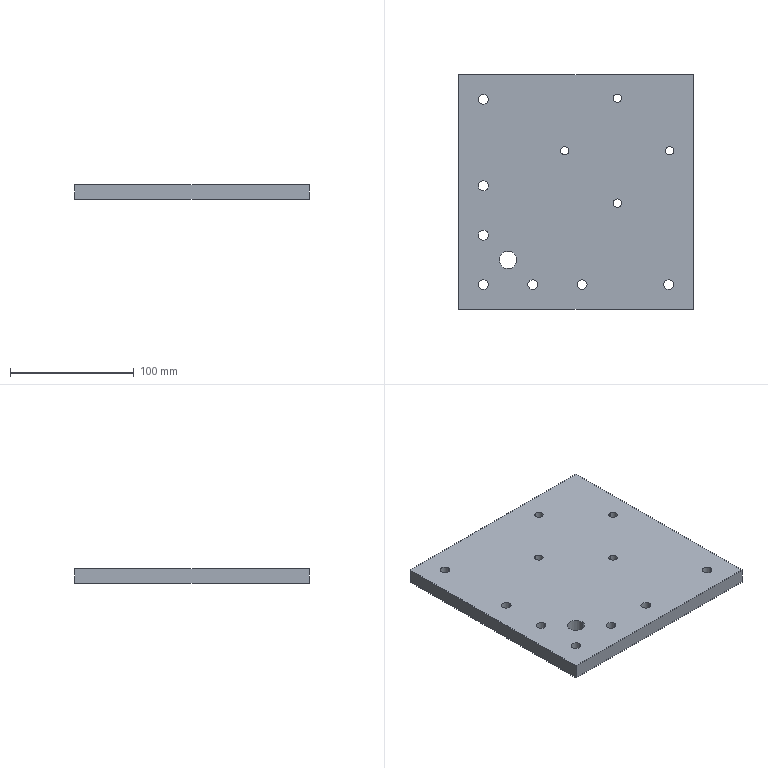Part | NX | 1 solid | 30 faces | box 190 x 190 x 12 mm | volume 425413 mm3 | cylinder 24 | plane 6 | commonest cylinder face diameters 8 x14 6.75 x8 14 x2
STEP:
#1=CARTESIAN_POINT('',(-95.,-95.,-6.));
#2=VERTEX_POINT('',#1);
#3=CARTESIAN_POINT('',(-95.,95.,-6.));
#4=VERTEX_POINT('',#3);
#5=CARTESIAN_POINT('',(-95.,-95.,-6.));
#6=DIRECTION('',(0.,1.,0.));
#7=VECTOR('',#6,1000.);
#8=LINE('',#5,#7);
#9=EDGE_CURVE('',#2,#4,#8,.T.);
#10=ORIENTED_EDGE('',*,*,#9,.T.);
#11=CARTESIAN_POINT('',(95.,95.,-6.));
#12=VERTEX_POINT('',#11);
#13=CARTESIAN_POINT('',(-95.,95.,-6.));
#14=DIRECTION('',(1.,0.,0.));
#15=VECTOR('',#14,1000.);
#16=LINE('',#13,#15);
#17=EDGE_CURVE('',#4,#12,#16,.T.);
#18=ORIENTED_EDGE('',*,*,#17,.T.);
#19=CARTESIAN_POINT('',(95.,-95.,-6.));
#20=VERTEX_POINT('',#19);
#21=CARTESIAN_POINT('',(95.,95.,-6.));
#22=DIRECTION('',(0.,-1.,0.));
#23=VECTOR('',#22,1000.);
#24=LINE('',#21,#23);
#25=EDGE_CURVE('',#12,#20,#24,.T.);
#26=ORIENTED_EDGE('',*,*,#25,.T.);
#27=CARTESIAN_POINT('',(95.,-95.,-6.));
#28=DIRECTION('',(-1.,0.,0.));
#29=VECTOR('',#28,1000.);
#30=LINE('',#27,#29);
#31=EDGE_CURVE('',#20,#2,#30,.T.);
#32=ORIENTED_EDGE('',*,*,#31,.T.);
#33=EDGE_LOOP('',(#10,#18,#26,#32));
#34=FACE_BOUND('',#33,.T.);
#35=CARTESIAN_POINT('',(1.,-75.,-6.));
#36=VERTEX_POINT('',#35);
#37=CARTESIAN_POINT('',(9.,-75.,-6.));
#38=VERTEX_POINT('',#37);
#39=CARTESIAN_POINT('',(5.,-75.,-6.));
#40=DIRECTION('',(0.,0.,-1.));
#41=DIRECTION('',(1.,0.,0.));
#42=AXIS2_PLACEMENT_3D('',#39,#40,#41);
#43=CIRCLE('',#42,4.);
#44=EDGE_CURVE('',#36,#38,#43,.T.);
#45=ORIENTED_EDGE('',*,*,#44,.F.);
#46=CARTESIAN_POINT('',(5.,-75.,-6.));
#47=DIRECTION('',(0.,0.,-1.));
#48=DIRECTION('',(1.,0.,0.));
#49=AXIS2_PLACEMENT_3D('',#46,#47,#48);
#50=CIRCLE('',#49,4.);
#51=EDGE_CURVE('',#38,#36,#50,.T.);
#52=ORIENTED_EDGE('',*,*,#51,.F.);
#53=EDGE_LOOP('',(#45,#52));
#54=FACE_BOUND('',#53,.T.);
#55=CARTESIAN_POINT('',(-79.,5.,-6.));
#56=VERTEX_POINT('',#55);
#57=CARTESIAN_POINT('',(-71.,5.,-6.));
#58=VERTEX_POINT('',#57);
#59=CARTESIAN_POINT('',(-75.,5.,-6.));
#60=DIRECTION('',(0.,0.,-1.));
#61=DIRECTION('',(1.,0.,0.));
#62=AXIS2_PLACEMENT_3D('',#59,#60,#61);
#63=CIRCLE('',#62,4.);
#64=EDGE_CURVE('',#56,#58,#63,.T.);
#65=ORIENTED_EDGE('',*,*,#64,.F.);
#66=CARTESIAN_POINT('',(-75.,5.,-6.));
#67=DIRECTION('',(0.,0.,-1.));
#68=DIRECTION('',(1.,0.,0.));
#69=AXIS2_PLACEMENT_3D('',#66,#67,#68);
#70=CIRCLE('',#69,4.);
#71=EDGE_CURVE('',#58,#56,#70,.T.);
#72=ORIENTED_EDGE('',*,*,#71,.F.);
#73=EDGE_LOOP('',(#65,#72));
#74=FACE_BOUND('',#73,.T.);
#75=CARTESIAN_POINT('',(-79.,-35.,-6.));
#76=VERTEX_POINT('',#75);
#77=CARTESIAN_POINT('',(-71.,-35.,-6.));
#78=VERTEX_POINT('',#77);
#79=CARTESIAN_POINT('',(-75.,-35.,-6.));
#80=DIRECTION('',(0.,0.,-1.));
#81=DIRECTION('',(1.,0.,0.));
#82=AXIS2_PLACEMENT_3D('',#79,#80,#81);
#83=CIRCLE('',#82,4.);
#84=EDGE_CURVE('',#76,#78,#83,.T.);
#85=ORIENTED_EDGE('',*,*,#84,.F.);
#86=CARTESIAN_POINT('',(-75.,-35.,-6.));
#87=DIRECTION('',(0.,0.,-1.));
#88=DIRECTION('',(1.,0.,0.));
#89=AXIS2_PLACEMENT_3D('',#86,#87,#88);
#90=CIRCLE('',#89,4.);
#91=EDGE_CURVE('',#78,#76,#90,.T.);
#92=ORIENTED_EDGE('',*,*,#91,.F.);
#93=EDGE_LOOP('',(#85,#92));
#94=FACE_BOUND('',#93,.T.);
#95=CARTESIAN_POINT('',(-79.,-75.,-6.));
#96=VERTEX_POINT('',#95);
#97=CARTESIAN_POINT('',(-71.,-75.,-6.));
#98=VERTEX_POINT('',#97);
#99=CARTESIAN_POINT('',(-75.,-75.,-6.));
#100=DIRECTION('',(0.,0.,-1.));
#101=DIRECTION('',(1.,0.,0.));
#102=AXIS2_PLACEMENT_3D('',#99,#100,#101);
#103=CIRCLE('',#102,4.);
#104=EDGE_CURVE('',#96,#98,#103,.T.);
#105=ORIENTED_EDGE('',*,*,#104,.F.);
#106=CARTESIAN_POINT('',(-75.,-75.,-6.));
#107=DIRECTION('',(0.,0.,-1.));
#108=DIRECTION('',(1.,0.,0.));
#109=AXIS2_PLACEMENT_3D('',#106,#107,#108);
#110=CIRCLE('',#109,4.);
#111=EDGE_CURVE('',#98,#96,#110,.T.);
#112=ORIENTED_EDGE('',*,*,#111,.F.);
#113=EDGE_LOOP('',(#105,#112));
#114=FACE_BOUND('',#113,.T.);
#115=CARTESIAN_POINT('',(-31.,-75.,-6.));
#116=VERTEX_POINT('',#115);
#117=CARTESIAN_POINT('',(-39.,-75.,-6.));
#118=VERTEX_POINT('',#117);
#119=CARTESIAN_POINT('',(-35.,-75.,-6.));
#120=DIRECTION('',(0.,0.,-1.));
#121=DIRECTION('',(1.,0.,0.));
#122=AXIS2_PLACEMENT_3D('',#119,#120,#121);
#123=CIRCLE('',#122,4.);
#124=EDGE_CURVE('',#116,#118,#123,.T.);
#125=ORIENTED_EDGE('',*,*,#124,.F.);
#126=CARTESIAN_POINT('',(-35.,-75.,-6.));
#127=DIRECTION('',(0.,0.,-1.));
#128=DIRECTION('',(1.,0.,0.));
#129=AXIS2_PLACEMENT_3D('',#126,#127,#128);
#130=CIRCLE('',#129,4.);
#131=EDGE_CURVE('',#118,#116,#130,.T.);
#132=ORIENTED_EDGE('',*,*,#131,.F.);
#133=EDGE_LOOP('',(#125,#132));
#134=FACE_BOUND('',#133,.T.);
#135=CARTESIAN_POINT('',(-71.,75.,-6.));
#136=VERTEX_POINT('',#135);
#137=CARTESIAN_POINT('',(-79.,75.,-6.));
#138=VERTEX_POINT('',#137);
#139=CARTESIAN_POINT('',(-75.,75.,-6.));
#140=DIRECTION('',(0.,0.,-1.));
#141=DIRECTION('',(1.,0.,0.));
#142=AXIS2_PLACEMENT_3D('',#139,#140,#141);
#143=CIRCLE('',#142,4.);
#144=EDGE_CURVE('',#136,#138,#143,.T.);
#145=ORIENTED_EDGE('',*,*,#144,.F.);
#146=CARTESIAN_POINT('',(-75.,75.,-6.));
#147=DIRECTION('',(0.,0.,-1.));
#148=DIRECTION('',(1.,0.,0.));
#149=AXIS2_PLACEMENT_3D('',#146,#147,#148);
#150=CIRCLE('',#149,4.);
#151=EDGE_CURVE('',#138,#136,#150,.T.);
#152=ORIENTED_EDGE('',*,*,#151,.F.);
#153=EDGE_LOOP('',(#145,#152));
#154=FACE_BOUND('',#153,.T.);
#155=CARTESIAN_POINT('',(71.,-75.,-6.));
#156=VERTEX_POINT('',#155);
#157=CARTESIAN_POINT('',(79.,-75.,-6.));
#158=VERTEX_POINT('',#157);
#159=CARTESIAN_POINT('',(75.,-75.,-6.));
#160=DIRECTION('',(0.,0.,-1.));
#161=DIRECTION('',(1.,0.,0.));
#162=AXIS2_PLACEMENT_3D('',#159,#160,#161);
#163=CIRCLE('',#162,4.);
#164=EDGE_CURVE('',#156,#158,#163,.T.);
#165=ORIENTED_EDGE('',*,*,#164,.F.);
#166=CARTESIAN_POINT('',(75.,-75.,-6.));
#167=DIRECTION('',(0.,0.,-1.));
#168=DIRECTION('',(1.,0.,0.));
#169=AXIS2_PLACEMENT_3D('',#166,#167,#168);
#170=CIRCLE('',#169,4.);
#171=EDGE_CURVE('',#158,#156,#170,.T.);
#172=ORIENTED_EDGE('',*,*,#171,.F.);
#173=EDGE_LOOP('',(#165,#172));
#174=FACE_BOUND('',#173,.T.);
#175=CARTESIAN_POINT('',(-48.,-55.,-6.));
#176=VERTEX_POINT('',#175);
#177=CARTESIAN_POINT('',(-62.,-55.,-6.));
#178=VERTEX_POINT('',#177);
#179=CARTESIAN_POINT('',(-55.,-55.,-6.));
#180=DIRECTION('',(0.,0.,-1.));
#181=DIRECTION('',(-1.,0.,0.));
#182=AXIS2_PLACEMENT_3D('',#179,#180,#181);
#183=CIRCLE('',#182,7.);
#184=EDGE_CURVE('',#176,#178,#183,.T.);
#185=ORIENTED_EDGE('',*,*,#184,.F.);
#186=CARTESIAN_POINT('',(-55.,-55.,-6.));
#187=DIRECTION('',(0.,0.,-1.));
#188=DIRECTION('',(-1.,0.,0.));
#189=AXIS2_PLACEMENT_3D('',#186,#187,#188);
#190=CIRCLE('',#189,7.);
#191=EDGE_CURVE('',#178,#176,#190,.T.);
#192=ORIENTED_EDGE('',*,*,#191,.F.);
#193=EDGE_LOOP('',(#185,#192));
#194=FACE_BOUND('',#193,.T.);
#195=CARTESIAN_POINT('',(-9.026,36.775,-6.));
#196=VERTEX_POINT('',#195);
#197=CARTESIAN_POINT('',(-9.026,30.025,-6.));
#198=VERTEX_POINT('',#197);
#199=CARTESIAN_POINT('',(-9.026,33.4,-6.));
#200=DIRECTION('',(0.,0.,-1.));
#201=DIRECTION('',(0.,1.,0.));
#202=AXIS2_PLACEMENT_3D('',#199,#200,#201);
#203=CIRCLE('',#202,3.375);
#204=EDGE_CURVE('',#196,#198,#203,.T.);
#205=ORIENTED_EDGE('',*,*,#204,.F.);
#206=CARTESIAN_POINT('',(-9.026,33.4,-6.));
#207=DIRECTION('',(0.,0.,-1.));
#208=DIRECTION('',(0.,1.,0.));
#209=AXIS2_PLACEMENT_3D('',#206,#207,#208);
#210=CIRCLE('',#209,3.375);
#211=EDGE_CURVE('',#198,#196,#210,.T.);
#212=ORIENTED_EDGE('',*,*,#211,.F.);
#213=EDGE_LOOP('',(#205,#212));
#214=FACE_BOUND('',#213,.T.);
#215=CARTESIAN_POINT('',(75.826,36.775,-6.));
#216=VERTEX_POINT('',#215);
#217=CARTESIAN_POINT('',(75.826,30.025,-6.));
#218=VERTEX_POINT('',#217);
#219=CARTESIAN_POINT('',(75.826,33.4,-6.));
#220=DIRECTION('',(0.,0.,-1.));
#221=DIRECTION('',(0.,1.,0.));
#222=AXIS2_PLACEMENT_3D('',#219,#220,#221);
#223=CIRCLE('',#222,3.375);
#224=EDGE_CURVE('',#216,#218,#223,.T.);
#225=ORIENTED_EDGE('',*,*,#224,.F.);
#226=CARTESIAN_POINT('',(75.826,33.4,-6.));
#227=DIRECTION('',(0.,0.,-1.));
#228=DIRECTION('',(0.,1.,0.));
#229=AXIS2_PLACEMENT_3D('',#226,#227,#228);
#230=CIRCLE('',#229,3.375);
#231=EDGE_CURVE('',#218,#216,#230,.T.);
#232=ORIENTED_EDGE('',*,*,#231,.F.);
#233=EDGE_LOOP('',(#225,#232));
#234=FACE_BOUND('',#233,.T.);
#235=CARTESIAN_POINT('',(33.4,72.451,-6.));
#236=VERTEX_POINT('',#235);
#237=CARTESIAN_POINT('',(33.4,79.201,-6.));
#238=VERTEX_POINT('',#237);
#239=CARTESIAN_POINT('',(33.4,75.826,-6.));
#240=DIRECTION('',(0.,0.,-1.));
#241=DIRECTION('',(0.,1.,0.));
#242=AXIS2_PLACEMENT_3D('',#239,#240,#241);
#243=CIRCLE('',#242,3.375);
#244=EDGE_CURVE('',#236,#238,#243,.T.);
#245=ORIENTED_EDGE('',*,*,#244,.F.);
#246=CARTESIAN_POINT('',(33.4,75.826,-6.));
#247=DIRECTION('',(0.,0.,-1.));
#248=DIRECTION('',(0.,1.,0.));
#249=AXIS2_PLACEMENT_3D('',#246,#247,#248);
#250=CIRCLE('',#249,3.375);
#251=EDGE_CURVE('',#238,#236,#250,.T.);
#252=ORIENTED_EDGE('',*,*,#251,.F.);
#253=EDGE_LOOP('',(#245,#252));
#254=FACE_BOUND('',#253,.T.);
#255=CARTESIAN_POINT('',(33.4,-12.401,-6.));
#256=VERTEX_POINT('',#255);
#257=CARTESIAN_POINT('',(33.4,-5.651,-6.));
#258=VERTEX_POINT('',#257);
#259=CARTESIAN_POINT('',(33.4,-9.026,-6.));
#260=DIRECTION('',(0.,0.,-1.));
#261=DIRECTION('',(0.,1.,0.));
#262=AXIS2_PLACEMENT_3D('',#259,#260,#261);
#263=CIRCLE('',#262,3.375);
#264=EDGE_CURVE('',#256,#258,#263,.T.);
#265=ORIENTED_EDGE('',*,*,#264,.F.);
#266=CARTESIAN_POINT('',(33.4,-9.026,-6.));
#267=DIRECTION('',(0.,0.,-1.));
#268=DIRECTION('',(0.,1.,0.));
#269=AXIS2_PLACEMENT_3D('',#266,#267,#268);
#270=CIRCLE('',#269,3.375);
#271=EDGE_CURVE('',#258,#256,#270,.T.);
#272=ORIENTED_EDGE('',*,*,#271,.F.);
#273=EDGE_LOOP('',(#265,#272));
#274=FACE_BOUND('',#273,.T.);
#275=CARTESIAN_POINT('',(0.,0.,-6.));
#276=DIRECTION('',(0.,0.,1.));
#277=DIRECTION('',(1.,0.,0.));
#278=AXIS2_PLACEMENT_3D('',#275,#276,#277);
#279=PLANE('',#278);
#280=ADVANCED_FACE('',(#34,#54,#74,#94,#114,#134,#154,#174,#194,#214,#234,#254,#274),#279,.F.);
#281=ORIENTED_EDGE('',*,*,#9,.F.);
#282=CARTESIAN_POINT('',(-95.,-95.,6.));
#283=VERTEX_POINT('',#282);
#284=CARTESIAN_POINT('',(-95.,-95.,6.));
#285=DIRECTION('',(0.,0.,-1.));
#286=VECTOR('',#285,1000.);
#287=LINE('',#284,#286);
#288=EDGE_CURVE('',#283,#2,#287,.T.);
#289=ORIENTED_EDGE('',*,*,#288,.F.);
#290=CARTESIAN_POINT('',(-95.,95.,6.));
#291=VERTEX_POINT('',#290);
#292=CARTESIAN_POINT('',(-95.,-95.,6.));
#293=DIRECTION('',(0.,1.,0.));
#294=VECTOR('',#293,1000.);
#295=LINE('',#292,#294);
#296=EDGE_CURVE('',#283,#291,#295,.T.);
#297=ORIENTED_EDGE('',*,*,#296,.T.);
#298=CARTESIAN_POINT('',(-95.,95.,6.));
#299=DIRECTION('',(0.,0.,-1.));
#300=VECTOR('',#299,1000.);
#301=LINE('',#298,#300);
#302=EDGE_CURVE('',#291,#4,#301,.T.);
#303=ORIENTED_EDGE('',*,*,#302,.T.);
#304=EDGE_LOOP('',(#281,#289,#297,#303));
#305=FACE_BOUND('',#304,.T.);
#306=CARTESIAN_POINT('',(-95.,95.,-6.));
#307=DIRECTION('',(-1.,0.,0.));
#308=DIRECTION('',(0.,0.,1.));
#309=AXIS2_PLACEMENT_3D('',#306,#307,#308);
#310=PLANE('',#309);
#311=ADVANCED_FACE('',(#305),#310,.T.);
#312=ORIENTED_EDGE('',*,*,#17,.F.);
#313=ORIENTED_EDGE('',*,*,#302,.F.);
#314=CARTESIAN_POINT('',(95.,95.,6.));
#315=VERTEX_POINT('',#314);
#316=CARTESIAN_POINT('',(-95.,95.,6.));
#317=DIRECTION('',(1.,0.,0.));
#318=VECTOR('',#317,1000.);
#319=LINE('',#316,#318);
#320=EDGE_CURVE('',#291,#315,#319,.T.);
#321=ORIENTED_EDGE('',*,*,#320,.T.);
#322=CARTESIAN_POINT('',(95.,95.,6.));
#323=DIRECTION('',(0.,0.,-1.));
#324=VECTOR('',#323,1000.);
#325=LINE('',#322,#324);
#326=EDGE_CURVE('',#315,#12,#325,.T.);
#327=ORIENTED_EDGE('',*,*,#326,.T.);
#328=EDGE_LOOP('',(#312,#313,#321,#327));
#329=FACE_BOUND('',#328,.T.);
#330=CARTESIAN_POINT('',(95.,95.,-6.));
#331=DIRECTION('',(0.,1.,0.));
#332=DIRECTION('',(1.,0.,0.));
#333=AXIS2_PLACEMENT_3D('',#330,#331,#332);
#334=PLANE('',#333);
#335=ADVANCED_FACE('',(#329),#334,.T.);
#336=ORIENTED_EDGE('',*,*,#25,.F.);
#337=ORIENTED_EDGE('',*,*,#326,.F.);
#338=CARTESIAN_POINT('',(95.,-95.,6.));
#339=VERTEX_POINT('',#338);
#340=CARTESIAN_POINT('',(95.,95.,6.));
#341=DIRECTION('',(0.,-1.,0.));
#342=VECTOR('',#341,1000.);
#343=LINE('',#340,#342);
#344=EDGE_CURVE('',#315,#339,#343,.T.);
#345=ORIENTED_EDGE('',*,*,#344,.T.);
#346=CARTESIAN_POINT('',(95.,-95.,6.));
#347=DIRECTION('',(0.,0.,-1.));
#348=VECTOR('',#347,1000.);
#349=LINE('',#346,#348);
#350=EDGE_CURVE('',#339,#20,#349,.T.);
#351=ORIENTED_EDGE('',*,*,#350,.T.);
#352=EDGE_LOOP('',(#336,#337,#345,#351));
#353=FACE_BOUND('',#352,.T.);
#354=CARTESIAN_POINT('',(95.,-95.,-6.));
#355=DIRECTION('',(1.,0.,0.));
#356=DIRECTION('',(0.,1.,0.));
#357=AXIS2_PLACEMENT_3D('',#354,#355,#356);
#358=PLANE('',#357);
#359=ADVANCED_FACE('',(#353),#358,.T.);
#360=ORIENTED_EDGE('',*,*,#31,.F.);
#361=ORIENTED_EDGE('',*,*,#350,.F.);
#362=CARTESIAN_POINT('',(95.,-95.,6.));
#363=DIRECTION('',(-1.,0.,0.));
#364=VECTOR('',#363,1000.);
#365=LINE('',#362,#364);
#366=EDGE_CURVE('',#339,#283,#365,.T.);
#367=ORIENTED_EDGE('',*,*,#366,.T.);
#368=ORIENTED_EDGE('',*,*,#288,.T.);
#369=EDGE_LOOP('',(#360,#361,#367,#368));
#370=FACE_BOUND('',#369,.T.);
#371=CARTESIAN_POINT('',(-95.,-95.,-6.));
#372=DIRECTION('',(0.,-1.,0.));
#373=DIRECTION('',(0.,0.,-1.));
#374=AXIS2_PLACEMENT_3D('',#371,#372,#373);
#375=PLANE('',#374);
#376=ADVANCED_FACE('',(#370),#375,.T.);
#377=ORIENTED_EDGE('',*,*,#296,.F.);
#378=ORIENTED_EDGE('',*,*,#366,.F.);
#379=ORIENTED_EDGE('',*,*,#344,.F.);
#380=ORIENTED_EDGE('',*,*,#320,.F.);
#381=EDGE_LOOP('',(#377,#378,#379,#380));
#382=FACE_BOUND('',#381,.T.);
#383=CARTESIAN_POINT('',(9.,-75.,6.));
#384=VERTEX_POINT('',#383);
#385=CARTESIAN_POINT('',(1.,-75.,6.));
#386=VERTEX_POINT('',#385);
#387=CARTESIAN_POINT('',(5.,-75.,6.));
#388=DIRECTION('',(0.,0.,1.));
#389=DIRECTION('',(-1.,0.,0.));
#390=AXIS2_PLACEMENT_3D('',#387,#388,#389);
#391=CIRCLE('',#390,4.);
#392=EDGE_CURVE('',#384,#386,#391,.T.);
#393=ORIENTED_EDGE('',*,*,#392,.F.);
#394=CARTESIAN_POINT('',(5.,-75.,6.));
#395=DIRECTION('',(0.,0.,1.));
#396=DIRECTION('',(-1.,0.,0.));
#397=AXIS2_PLACEMENT_3D('',#394,#395,#396);
#398=CIRCLE('',#397,4.);
#399=EDGE_CURVE('',#386,#384,#398,.T.);
#400=ORIENTED_EDGE('',*,*,#399,.F.);
#401=EDGE_LOOP('',(#393,#400));
#402=FACE_BOUND('',#401,.T.);
#403=CARTESIAN_POINT('',(-71.,5.,6.));
#404=VERTEX_POINT('',#403);
#405=CARTESIAN_POINT('',(-79.,5.,6.));
#406=VERTEX_POINT('',#405);
#407=CARTESIAN_POINT('',(-75.,5.,6.));
#408=DIRECTION('',(0.,0.,1.));
#409=DIRECTION('',(-1.,0.,0.));
#410=AXIS2_PLACEMENT_3D('',#407,#408,#409);
#411=CIRCLE('',#410,4.);
#412=EDGE_CURVE('',#404,#406,#411,.T.);
#413=ORIENTED_EDGE('',*,*,#412,.F.);
#414=CARTESIAN_POINT('',(-75.,5.,6.));
#415=DIRECTION('',(0.,0.,1.));
#416=DIRECTION('',(-1.,0.,0.));
#417=AXIS2_PLACEMENT_3D('',#414,#415,#416);
#418=CIRCLE('',#417,4.);
#419=EDGE_CURVE('',#406,#404,#418,.T.);
#420=ORIENTED_EDGE('',*,*,#419,.F.);
#421=EDGE_LOOP('',(#413,#420));
#422=FACE_BOUND('',#421,.T.);
#423=CARTESIAN_POINT('',(-79.,-35.,6.));
#424=VERTEX_POINT('',#423);
#425=CARTESIAN_POINT('',(-71.,-35.,6.));
#426=VERTEX_POINT('',#425);
#427=CARTESIAN_POINT('',(-75.,-35.,6.));
#428=DIRECTION('',(0.,0.,1.));
#429=DIRECTION('',(-1.,0.,0.));
#430=AXIS2_PLACEMENT_3D('',#427,#428,#429);
#431=CIRCLE('',#430,4.);
#432=EDGE_CURVE('',#424,#426,#431,.T.);
#433=ORIENTED_EDGE('',*,*,#432,.F.);
#434=CARTESIAN_POINT('',(-75.,-35.,6.));
#435=DIRECTION('',(0.,0.,1.));
#436=DIRECTION('',(-1.,0.,0.));
#437=AXIS2_PLACEMENT_3D('',#434,#435,#436);
#438=CIRCLE('',#437,4.);
#439=EDGE_CURVE('',#426,#424,#438,.T.);
#440=ORIENTED_EDGE('',*,*,#439,.F.);
#441=EDGE_LOOP('',(#433,#440));
#442=FACE_BOUND('',#441,.T.);
#443=CARTESIAN_POINT('',(-79.,-75.,6.));
#444=VERTEX_POINT('',#443);
#445=CARTESIAN_POINT('',(-71.,-75.,6.));
#446=VERTEX_POINT('',#445);
#447=CARTESIAN_POINT('',(-75.,-75.,6.));
#448=DIRECTION('',(0.,0.,1.));
#449=DIRECTION('',(-1.,0.,0.));
#450=AXIS2_PLACEMENT_3D('',#447,#448,#449);
#451=CIRCLE('',#450,4.);
#452=EDGE_CURVE('',#444,#446,#451,.T.);
#453=ORIENTED_EDGE('',*,*,#452,.F.);
#454=CARTESIAN_POINT('',(-75.,-75.,6.));
#455=DIRECTION('',(0.,0.,1.));
#456=DIRECTION('',(-1.,0.,0.));
#457=AXIS2_PLACEMENT_3D('',#454,#455,#456);
#458=CIRCLE('',#457,4.);
#459=EDGE_CURVE('',#446,#444,#458,.T.);
#460=ORIENTED_EDGE('',*,*,#459,.F.);
#461=EDGE_LOOP('',(#453,#460));
#462=FACE_BOUND('',#461,.T.);
#463=CARTESIAN_POINT('',(-31.,-75.,6.));
#464=VERTEX_POINT('',#463);
#465=CARTESIAN_POINT('',(-39.,-75.,6.));
#466=VERTEX_POINT('',#465);
#467=CARTESIAN_POINT('',(-35.,-75.,6.));
#468=DIRECTION('',(0.,0.,1.));
#469=DIRECTION('',(-1.,0.,0.));
#470=AXIS2_PLACEMENT_3D('',#467,#468,#469);
#471=CIRCLE('',#470,4.);
#472=EDGE_CURVE('',#464,#466,#471,.T.);
#473=ORIENTED_EDGE('',*,*,#472,.F.);
#474=CARTESIAN_POINT('',(-35.,-75.,6.));
#475=DIRECTION('',(0.,0.,1.));
#476=DIRECTION('',(-1.,0.,0.));
#477=AXIS2_PLACEMENT_3D('',#474,#475,#476);
#478=CIRCLE('',#477,4.);
#479=EDGE_CURVE('',#466,#464,#478,.T.);
#480=ORIENTED_EDGE('',*,*,#479,.F.);
#481=EDGE_LOOP('',(#473,#480));
#482=FACE_BOUND('',#481,.T.);
#483=CARTESIAN_POINT('',(-79.,75.,6.));
#484=VERTEX_POINT('',#483);
#485=CARTESIAN_POINT('',(-71.,75.,6.));
#486=VERTEX_POINT('',#485);
#487=CARTESIAN_POINT('',(-75.,75.,6.));
#488=DIRECTION('',(0.,0.,1.));
#489=DIRECTION('',(-1.,0.,0.));
#490=AXIS2_PLACEMENT_3D('',#487,#488,#489);
#491=CIRCLE('',#490,4.);
#492=EDGE_CURVE('',#484,#486,#491,.T.);
#493=ORIENTED_EDGE('',*,*,#492,.F.);
#494=CARTESIAN_POINT('',(-75.,75.,6.));
#495=DIRECTION('',(0.,0.,1.));
#496=DIRECTION('',(-1.,0.,0.));
#497=AXIS2_PLACEMENT_3D('',#494,#495,#496);
#498=CIRCLE('',#497,4.);
#499=EDGE_CURVE('',#486,#484,#498,.T.);
#500=ORIENTED_EDGE('',*,*,#499,.F.);
#501=EDGE_LOOP('',(#493,#500));
#502=FACE_BOUND('',#501,.T.);
#503=CARTESIAN_POINT('',(79.,-75.,6.));
#504=VERTEX_POINT('',#503);
#505=CARTESIAN_POINT('',(71.,-75.,6.));
#506=VERTEX_POINT('',#505);
#507=CARTESIAN_POINT('',(75.,-75.,6.));
#508=DIRECTION('',(0.,0.,1.));
#509=DIRECTION('',(-1.,0.,0.));
#510=AXIS2_PLACEMENT_3D('',#507,#508,#509);
#511=CIRCLE('',#510,4.);
#512=EDGE_CURVE('',#504,#506,#511,.T.);
#513=ORIENTED_EDGE('',*,*,#512,.F.);
#514=CARTESIAN_POINT('',(75.,-75.,6.));
#515=DIRECTION('',(0.,0.,1.));
#516=DIRECTION('',(-1.,0.,0.));
#517=AXIS2_PLACEMENT_3D('',#514,#515,#516);
#518=CIRCLE('',#517,4.);
#519=EDGE_CURVE('',#506,#504,#518,.T.);
#520=ORIENTED_EDGE('',*,*,#519,.F.);
#521=EDGE_LOOP('',(#513,#520));
#522=FACE_BOUND('',#521,.T.);
#523=CARTESIAN_POINT('',(-48.,-55.,6.));
#524=VERTEX_POINT('',#523);
#525=CARTESIAN_POINT('',(-62.,-55.,6.));
#526=VERTEX_POINT('',#525);
#527=CARTESIAN_POINT('',(-55.,-55.,6.));
#528=DIRECTION('',(0.,0.,1.));
#529=DIRECTION('',(1.,0.,0.));
#530=AXIS2_PLACEMENT_3D('',#527,#528,#529);
#531=CIRCLE('',#530,7.);
#532=EDGE_CURVE('',#524,#526,#531,.T.);
#533=ORIENTED_EDGE('',*,*,#532,.F.);
#534=CARTESIAN_POINT('',(-55.,-55.,6.));
#535=DIRECTION('',(0.,0.,1.));
#536=DIRECTION('',(1.,0.,0.));
#537=AXIS2_PLACEMENT_3D('',#534,#535,#536);
#538=CIRCLE('',#537,7.);
#539=EDGE_CURVE('',#526,#524,#538,.T.);
#540=ORIENTED_EDGE('',*,*,#539,.F.);
#541=EDGE_LOOP('',(#533,#540));
#542=FACE_BOUND('',#541,.T.);
#543=CARTESIAN_POINT('',(-9.026,30.025,6.));
#544=VERTEX_POINT('',#543);
#545=CARTESIAN_POINT('',(-9.026,36.775,6.));
#546=VERTEX_POINT('',#545);
#547=CARTESIAN_POINT('',(-9.026,33.4,6.));
#548=DIRECTION('',(0.,0.,1.));
#549=DIRECTION('',(0.,-1.,0.));
#550=AXIS2_PLACEMENT_3D('',#547,#548,#549);
#551=CIRCLE('',#550,3.375);
#552=EDGE_CURVE('',#544,#546,#551,.T.);
#553=ORIENTED_EDGE('',*,*,#552,.F.);
#554=CARTESIAN_POINT('',(-9.026,33.4,6.));
#555=DIRECTION('',(0.,0.,1.));
#556=DIRECTION('',(0.,-1.,0.));
#557=AXIS2_PLACEMENT_3D('',#554,#555,#556);
#558=CIRCLE('',#557,3.375);
#559=EDGE_CURVE('',#546,#544,#558,.T.);
#560=ORIENTED_EDGE('',*,*,#559,.F.);
#561=EDGE_LOOP('',(#553,#560));
#562=FACE_BOUND('',#561,.T.);
#563=CARTESIAN_POINT('',(75.826,30.025,6.));
#564=VERTEX_POINT('',#563);
#565=CARTESIAN_POINT('',(75.826,36.775,6.));
#566=VERTEX_POINT('',#565);
#567=CARTESIAN_POINT('',(75.826,33.4,6.));
#568=DIRECTION('',(0.,0.,1.));
#569=DIRECTION('',(0.,-1.,0.));
#570=AXIS2_PLACEMENT_3D('',#567,#568,#569);
#571=CIRCLE('',#570,3.375);
#572=EDGE_CURVE('',#564,#566,#571,.T.);
#573=ORIENTED_EDGE('',*,*,#572,.F.);
#574=CARTESIAN_POINT('',(75.826,33.4,6.));
#575=DIRECTION('',(0.,0.,1.));
#576=DIRECTION('',(0.,-1.,0.));
#577=AXIS2_PLACEMENT_3D('',#574,#575,#576);
#578=CIRCLE('',#577,3.375);
#579=EDGE_CURVE('',#566,#564,#578,.T.);
#580=ORIENTED_EDGE('',*,*,#579,.F.);
#581=EDGE_LOOP('',(#573,#580));
#582=FACE_BOUND('',#581,.T.);
#583=CARTESIAN_POINT('',(33.4,72.451,6.));
#584=VERTEX_POINT('',#583);
#585=CARTESIAN_POINT('',(33.4,79.201,6.));
#586=VERTEX_POINT('',#585);
#587=CARTESIAN_POINT('',(33.4,75.826,6.));
#588=DIRECTION('',(0.,0.,1.));
#589=DIRECTION('',(0.,-1.,0.));
#590=AXIS2_PLACEMENT_3D('',#587,#588,#589);
#591=CIRCLE('',#590,3.375);
#592=EDGE_CURVE('',#584,#586,#591,.T.);
#593=ORIENTED_EDGE('',*,*,#592,.F.);
#594=CARTESIAN_POINT('',(33.4,75.826,6.));
#595=DIRECTION('',(0.,0.,1.));
#596=DIRECTION('',(0.,-1.,0.));
#597=AXIS2_PLACEMENT_3D('',#594,#595,#596);
#598=CIRCLE('',#597,3.375);
#599=EDGE_CURVE('',#586,#584,#598,.T.);
#600=ORIENTED_EDGE('',*,*,#599,.F.);
#601=EDGE_LOOP('',(#593,#600));
#602=FACE_BOUND('',#601,.T.);
#603=CARTESIAN_POINT('',(33.4,-5.651,6.));
#604=VERTEX_POINT('',#603);
#605=CARTESIAN_POINT('',(33.4,-12.401,6.));
#606=VERTEX_POINT('',#605);
#607=CARTESIAN_POINT('',(33.4,-9.026,6.));
#608=DIRECTION('',(0.,0.,1.));
#609=DIRECTION('',(0.,-1.,0.));
#610=AXIS2_PLACEMENT_3D('',#607,#608,#609);
#611=CIRCLE('',#610,3.375);
#612=EDGE_CURVE('',#604,#606,#611,.T.);
#613=ORIENTED_EDGE('',*,*,#612,.F.);
#614=CARTESIAN_POINT('',(33.4,-9.026,6.));
#615=DIRECTION('',(0.,0.,1.));
#616=DIRECTION('',(0.,-1.,0.));
#617=AXIS2_PLACEMENT_3D('',#614,#615,#616);
#618=CIRCLE('',#617,3.375);
#619=EDGE_CURVE('',#606,#604,#618,.T.);
#620=ORIENTED_EDGE('',*,*,#619,.F.);
#621=EDGE_LOOP('',(#613,#620));
#622=FACE_BOUND('',#621,.T.);
#623=CARTESIAN_POINT('',(0.,0.,6.));
#624=DIRECTION('',(0.,0.,1.));
#625=DIRECTION('',(1.,0.,0.));
#626=AXIS2_PLACEMENT_3D('',#623,#624,#625);
#627=PLANE('',#626);
#628=ADVANCED_FACE('',(#382,#402,#422,#442,#462,#482,#502,#522,#542,#562,#582,#602,#622),#627,.T.);
#629=ORIENTED_EDGE('',*,*,#392,.T.);
#630=CARTESIAN_POINT('',(1.,-75.,6.));
#631=DIRECTION('',(0.,0.,-1.));
#632=VECTOR('',#631,1000.);
#633=LINE('',#630,#632);
#634=EDGE_CURVE('',#36,#386,#633,.F.);
#635=ORIENTED_EDGE('',*,*,#634,.F.);
#636=ORIENTED_EDGE('',*,*,#44,.T.);
#637=CARTESIAN_POINT('',(9.,-75.,6.));
#638=DIRECTION('',(0.,0.,-1.));
#639=VECTOR('',#638,1000.);
#640=LINE('',#637,#639);
#641=EDGE_CURVE('',#38,#384,#640,.F.);
#642=ORIENTED_EDGE('',*,*,#641,.T.);
#643=EDGE_LOOP('',(#629,#635,#636,#642));
#644=FACE_BOUND('',#643,.T.);
#645=CARTESIAN_POINT('',(5.,-75.,6.));
#646=DIRECTION('',(0.,0.,-1.));
#647=DIRECTION('',(-1.,0.,0.));
#648=AXIS2_PLACEMENT_3D('',#645,#646,#647);
#649=CYLINDRICAL_SURFACE('',#648,4.);
#650=ADVANCED_FACE('',(#644),#649,.F.);
#651=ORIENTED_EDGE('',*,*,#264,.T.);
#652=CARTESIAN_POINT('',(33.4,-5.651,6.));
#653=DIRECTION('',(0.,0.,1.));
#654=VECTOR('',#653,1000.);
#655=LINE('',#652,#654);
#656=EDGE_CURVE('',#258,#604,#655,.T.);
#657=ORIENTED_EDGE('',*,*,#656,.T.);
#658=ORIENTED_EDGE('',*,*,#612,.T.);
#659=CARTESIAN_POINT('',(33.4,-12.401,6.));
#660=DIRECTION('',(0.,0.,1.));
#661=VECTOR('',#660,1000.);
#662=LINE('',#659,#661);
#663=EDGE_CURVE('',#256,#606,#662,.T.);
#664=ORIENTED_EDGE('',*,*,#663,.F.);
#665=EDGE_LOOP('',(#651,#657,#658,#664));
#666=FACE_BOUND('',#665,.T.);
#667=CARTESIAN_POINT('',(33.4,-9.026,6.));
#668=DIRECTION('',(0.,0.,1.));
#669=DIRECTION('',(0.,1.,0.));
#670=AXIS2_PLACEMENT_3D('',#667,#668,#669);
#671=CYLINDRICAL_SURFACE('',#670,3.375);
#672=ADVANCED_FACE('',(#666),#671,.F.);
#673=ORIENTED_EDGE('',*,*,#64,.T.);
#674=CARTESIAN_POINT('',(-71.,5.,6.));
#675=DIRECTION('',(0.,0.,-1.));
#676=VECTOR('',#675,1000.);
#677=LINE('',#674,#676);
#678=EDGE_CURVE('',#58,#404,#677,.F.);
#679=ORIENTED_EDGE('',*,*,#678,.T.);
#680=ORIENTED_EDGE('',*,*,#412,.T.);
#681=CARTESIAN_POINT('',(-79.,5.,6.));
#682=DIRECTION('',(0.,0.,-1.));
#683=VECTOR('',#682,1000.);
#684=LINE('',#681,#683);
#685=EDGE_CURVE('',#56,#406,#684,.F.);
#686=ORIENTED_EDGE('',*,*,#685,.F.);
#687=EDGE_LOOP('',(#673,#679,#680,#686));
#688=FACE_BOUND('',#687,.T.);
#689=CARTESIAN_POINT('',(-75.,5.,6.));
#690=DIRECTION('',(0.,0.,-1.));
#691=DIRECTION('',(-1.,0.,0.));
#692=AXIS2_PLACEMENT_3D('',#689,#690,#691);
#693=CYLINDRICAL_SURFACE('',#692,4.);
#694=ADVANCED_FACE('',(#688),#693,.F.);
#695=ORIENTED_EDGE('',*,*,#552,.T.);
#696=CARTESIAN_POINT('',(-9.026,36.775,6.));
#697=DIRECTION('',(0.,0.,1.));
#698=VECTOR('',#697,1000.);
#699=LINE('',#696,#698);
#700=EDGE_CURVE('',#196,#546,#699,.T.);
#701=ORIENTED_EDGE('',*,*,#700,.F.);
#702=ORIENTED_EDGE('',*,*,#204,.T.);
#703=CARTESIAN_POINT('',(-9.026,30.025,6.));
#704=DIRECTION('',(0.,0.,1.));
#705=VECTOR('',#704,1000.);
#706=LINE('',#703,#705);
#707=EDGE_CURVE('',#198,#544,#706,.T.);
#708=ORIENTED_EDGE('',*,*,#707,.T.);
#709=EDGE_LOOP('',(#695,#701,#702,#708));
#710=FACE_BOUND('',#709,.T.);
#711=CARTESIAN_POINT('',(-9.026,33.4,6.));
#712=DIRECTION('',(0.,0.,1.));
#713=DIRECTION('',(0.,1.,0.));
#714=AXIS2_PLACEMENT_3D('',#711,#712,#713);
#715=CYLINDRICAL_SURFACE('',#714,3.375);
#716=ADVANCED_FACE('',(#710),#715,.F.);
#717=ORIENTED_EDGE('',*,*,#84,.T.);
#718=CARTESIAN_POINT('',(-71.,-35.,6.));
#719=DIRECTION('',(0.,0.,-1.));
#720=VECTOR('',#719,1000.);
#721=LINE('',#718,#720);
#722=EDGE_CURVE('',#426,#78,#721,.T.);
#723=ORIENTED_EDGE('',*,*,#722,.F.);
#724=ORIENTED_EDGE('',*,*,#439,.T.);
#725=CARTESIAN_POINT('',(-79.,-35.,6.));
#726=DIRECTION('',(0.,0.,-1.));
#727=VECTOR('',#726,1000.);
#728=LINE('',#725,#727);
#729=EDGE_CURVE('',#424,#76,#728,.T.);
#730=ORIENTED_EDGE('',*,*,#729,.T.);
#731=EDGE_LOOP('',(#717,#723,#724,#730));
#732=FACE_BOUND('',#731,.T.);
#733=CARTESIAN_POINT('',(-75.,-35.,6.));
#734=DIRECTION('',(0.,0.,-1.));
#735=DIRECTION('',(-1.,0.,0.));
#736=AXIS2_PLACEMENT_3D('',#733,#734,#735);
#737=CYLINDRICAL_SURFACE('',#736,4.);
#738=ADVANCED_FACE('',(#732),#737,.F.);
#739=ORIENTED_EDGE('',*,*,#244,.T.);
#740=CARTESIAN_POINT('',(33.4,79.201,6.));
#741=DIRECTION('',(0.,0.,1.));
#742=VECTOR('',#741,1000.);
#743=LINE('',#740,#742);
#744=EDGE_CURVE('',#238,#586,#743,.T.);
#745=ORIENTED_EDGE('',*,*,#744,.T.);
#746=ORIENTED_EDGE('',*,*,#599,.T.);
#747=CARTESIAN_POINT('',(33.4,72.451,6.));
#748=DIRECTION('',(0.,0.,1.));
#749=VECTOR('',#748,1000.);
#750=LINE('',#747,#749);
#751=EDGE_CURVE('',#236,#584,#750,.T.);
#752=ORIENTED_EDGE('',*,*,#751,.F.);
#753=EDGE_LOOP('',(#739,#745,#746,#752));
#754=FACE_BOUND('',#753,.T.);
#755=CARTESIAN_POINT('',(33.4,75.826,6.));
#756=DIRECTION('',(0.,0.,1.));
#757=DIRECTION('',(0.,1.,0.));
#758=AXIS2_PLACEMENT_3D('',#755,#756,#757);
#759=CYLINDRICAL_SURFACE('',#758,3.375);
#760=ADVANCED_FACE('',(#754),#759,.F.);
#761=ORIENTED_EDGE('',*,*,#104,.T.);
#762=CARTESIAN_POINT('',(-71.,-75.,6.));
#763=DIRECTION('',(0.,0.,-1.));
#764=VECTOR('',#763,1000.);
#765=LINE('',#762,#764);
#766=EDGE_CURVE('',#446,#98,#765,.T.);
#767=ORIENTED_EDGE('',*,*,#766,.F.);
#768=ORIENTED_EDGE('',*,*,#459,.T.);
#769=CARTESIAN_POINT('',(-79.,-75.,6.));
#770=DIRECTION('',(0.,0.,-1.));
#771=VECTOR('',#770,1000.);
#772=LINE('',#769,#771);
#773=EDGE_CURVE('',#444,#96,#772,.T.);
#774=ORIENTED_EDGE('',*,*,#773,.T.);
#775=EDGE_LOOP('',(#761,#767,#768,#774));
#776=FACE_BOUND('',#775,.T.);
#777=CARTESIAN_POINT('',(-75.,-75.,6.));
#778=DIRECTION('',(0.,0.,-1.));
#779=DIRECTION('',(-1.,0.,0.));
#780=AXIS2_PLACEMENT_3D('',#777,#778,#779);
#781=CYLINDRICAL_SURFACE('',#780,4.);
#782=ADVANCED_FACE('',(#776),#781,.F.);
#783=ORIENTED_EDGE('',*,*,#572,.T.);
#784=CARTESIAN_POINT('',(75.826,36.775,6.));
#785=DIRECTION('',(0.,0.,1.));
#786=VECTOR('',#785,1000.);
#787=LINE('',#784,#786);
#788=EDGE_CURVE('',#216,#566,#787,.T.);
#789=ORIENTED_EDGE('',*,*,#788,.F.);
#790=ORIENTED_EDGE('',*,*,#224,.T.);
#791=CARTESIAN_POINT('',(75.826,30.025,6.));
#792=DIRECTION('',(0.,0.,1.));
#793=VECTOR('',#792,1000.);
#794=LINE('',#791,#793);
#795=EDGE_CURVE('',#218,#564,#794,.T.);
#796=ORIENTED_EDGE('',*,*,#795,.T.);
#797=EDGE_LOOP('',(#783,#789,#790,#796));
#798=FACE_BOUND('',#797,.T.);
#799=CARTESIAN_POINT('',(75.826,33.4,6.));
#800=DIRECTION('',(0.,0.,1.));
#801=DIRECTION('',(0.,1.,0.));
#802=AXIS2_PLACEMENT_3D('',#799,#800,#801);
#803=CYLINDRICAL_SURFACE('',#802,3.375);
#804=ADVANCED_FACE('',(#798),#803,.F.);
#805=ORIENTED_EDGE('',*,*,#472,.T.);
#806=CARTESIAN_POINT('',(-39.,-75.,6.));
#807=DIRECTION('',(0.,0.,-1.));
#808=VECTOR('',#807,1000.);
#809=LINE('',#806,#808);
#810=EDGE_CURVE('',#118,#466,#809,.F.);
#811=ORIENTED_EDGE('',*,*,#810,.F.);
#812=ORIENTED_EDGE('',*,*,#131,.T.);
#813=CARTESIAN_POINT('',(-31.,-75.,6.));
#814=DIRECTION('',(0.,0.,-1.));
#815=VECTOR('',#814,1000.);
#816=LINE('',#813,#815);
#817=EDGE_CURVE('',#116,#464,#816,.F.);
#818=ORIENTED_EDGE('',*,*,#817,.T.);
#819=EDGE_LOOP('',(#805,#811,#812,#818));
#820=FACE_BOUND('',#819,.T.);
#821=CARTESIAN_POINT('',(-35.,-75.,6.));
#822=DIRECTION('',(0.,0.,-1.));
#823=DIRECTION('',(-1.,0.,0.));
#824=AXIS2_PLACEMENT_3D('',#821,#822,#823);
#825=CYLINDRICAL_SURFACE('',#824,4.);
#826=ADVANCED_FACE('',(#820),#825,.F.);
#827=ORIENTED_EDGE('',*,*,#184,.T.);
#828=CARTESIAN_POINT('',(-62.,-55.,-7.86));
#829=DIRECTION('',(0.,0.,1.));
#830=VECTOR('',#829,1000.);
#831=LINE('',#828,#830);
#832=EDGE_CURVE('',#526,#178,#831,.F.);
#833=ORIENTED_EDGE('',*,*,#832,.F.);
#834=ORIENTED_EDGE('',*,*,#539,.T.);
#835=CARTESIAN_POINT('',(-48.,-55.,-7.86));
#836=DIRECTION('',(0.,0.,1.));
#837=VECTOR('',#836,1000.);
#838=LINE('',#835,#837);
#839=EDGE_CURVE('',#524,#176,#838,.F.);
#840=ORIENTED_EDGE('',*,*,#839,.T.);
#841=EDGE_LOOP('',(#827,#833,#834,#840));
#842=FACE_BOUND('',#841,.T.);
#843=CARTESIAN_POINT('',(-55.,-55.,-7.86));
#844=DIRECTION('',(0.,0.,1.));
#845=DIRECTION('',(-1.,0.,0.));
#846=AXIS2_PLACEMENT_3D('',#843,#844,#845);
#847=CYLINDRICAL_SURFACE('',#846,7.);
#848=ADVANCED_FACE('',(#842),#847,.F.);
#849=ORIENTED_EDGE('',*,*,#144,.T.);
#850=CARTESIAN_POINT('',(-79.,75.,6.));
#851=DIRECTION('',(0.,0.,-1.));
#852=VECTOR('',#851,1000.);
#853=LINE('',#850,#852);
#854=EDGE_CURVE('',#138,#484,#853,.F.);
#855=ORIENTED_EDGE('',*,*,#854,.T.);
#856=ORIENTED_EDGE('',*,*,#492,.T.);
#857=CARTESIAN_POINT('',(-71.,75.,6.));
#858=DIRECTION('',(0.,0.,-1.));
#859=VECTOR('',#858,1000.);
#860=LINE('',#857,#859);
#861=EDGE_CURVE('',#136,#486,#860,.F.);
#862=ORIENTED_EDGE('',*,*,#861,.F.);
#863=EDGE_LOOP('',(#849,#855,#856,#862));
#864=FACE_BOUND('',#863,.T.);
#865=CARTESIAN_POINT('',(-75.,75.,6.));
#866=DIRECTION('',(0.,0.,-1.));
#867=DIRECTION('',(-1.,0.,0.));
#868=AXIS2_PLACEMENT_3D('',#865,#866,#867);
#869=CYLINDRICAL_SURFACE('',#868,4.);
#870=ADVANCED_FACE('',(#864),#869,.F.);
#871=ORIENTED_EDGE('',*,*,#164,.T.);
#872=CARTESIAN_POINT('',(79.,-75.,6.));
#873=DIRECTION('',(0.,0.,-1.));
#874=VECTOR('',#873,1000.);
#875=LINE('',#872,#874);
#876=EDGE_CURVE('',#158,#504,#875,.F.);
#877=ORIENTED_EDGE('',*,*,#876,.T.);
#878=ORIENTED_EDGE('',*,*,#512,.T.);
#879=CARTESIAN_POINT('',(71.,-75.,6.));
#880=DIRECTION('',(0.,0.,-1.));
#881=VECTOR('',#880,1000.);
#882=LINE('',#879,#881);
#883=EDGE_CURVE('',#156,#506,#882,.F.);
#884=ORIENTED_EDGE('',*,*,#883,.F.);
#885=EDGE_LOOP('',(#871,#877,#878,#884));
#886=FACE_BOUND('',#885,.T.);
#887=CARTESIAN_POINT('',(75.,-75.,6.));
#888=DIRECTION('',(0.,0.,-1.));
#889=DIRECTION('',(-1.,0.,0.));
#890=AXIS2_PLACEMENT_3D('',#887,#888,#889);
#891=CYLINDRICAL_SURFACE('',#890,4.);
#892=ADVANCED_FACE('',(#886),#891,.F.);
#893=ORIENTED_EDGE('',*,*,#685,.T.);
#894=ORIENTED_EDGE('',*,*,#419,.T.);
#895=ORIENTED_EDGE('',*,*,#678,.F.);
#896=ORIENTED_EDGE('',*,*,#71,.T.);
#897=EDGE_LOOP('',(#893,#894,#895,#896));
#898=FACE_BOUND('',#897,.T.);
#899=CARTESIAN_POINT('',(-75.,5.,6.));
#900=DIRECTION('',(0.,0.,-1.));
#901=DIRECTION('',(-1.,0.,0.));
#902=AXIS2_PLACEMENT_3D('',#899,#900,#901);
#903=CYLINDRICAL_SURFACE('',#902,4.);
#904=ADVANCED_FACE('',(#898),#903,.F.);
#905=ORIENTED_EDGE('',*,*,#656,.F.);
#906=ORIENTED_EDGE('',*,*,#271,.T.);
#907=ORIENTED_EDGE('',*,*,#663,.T.);
#908=ORIENTED_EDGE('',*,*,#619,.T.);
#909=EDGE_LOOP('',(#905,#906,#907,#908));
#910=FACE_BOUND('',#909,.T.);
#911=CARTESIAN_POINT('',(33.4,-9.026,6.));
#912=DIRECTION('',(0.,0.,1.));
#913=DIRECTION('',(0.,1.,0.));
#914=AXIS2_PLACEMENT_3D('',#911,#912,#913);
#915=CYLINDRICAL_SURFACE('',#914,3.375);
#916=ADVANCED_FACE('',(#910),#915,.F.);
#917=ORIENTED_EDGE('',*,*,#700,.T.);
#918=ORIENTED_EDGE('',*,*,#559,.T.);
#919=ORIENTED_EDGE('',*,*,#707,.F.);
#920=ORIENTED_EDGE('',*,*,#211,.T.);
#921=EDGE_LOOP('',(#917,#918,#919,#920));
#922=FACE_BOUND('',#921,.T.);
#923=CARTESIAN_POINT('',(-9.026,33.4,6.));
#924=DIRECTION('',(0.,0.,1.));
#925=DIRECTION('',(0.,1.,0.));
#926=AXIS2_PLACEMENT_3D('',#923,#924,#925);
#927=CYLINDRICAL_SURFACE('',#926,3.375);
#928=ADVANCED_FACE('',(#922),#927,.F.);
#929=ORIENTED_EDGE('',*,*,#854,.F.);
#930=ORIENTED_EDGE('',*,*,#151,.T.);
#931=ORIENTED_EDGE('',*,*,#861,.T.);
#932=ORIENTED_EDGE('',*,*,#499,.T.);
#933=EDGE_LOOP('',(#929,#930,#931,#932));
#934=FACE_BOUND('',#933,.T.);
#935=CARTESIAN_POINT('',(-75.,75.,6.));
#936=DIRECTION('',(0.,0.,-1.));
#937=DIRECTION('',(-1.,0.,0.));
#938=AXIS2_PLACEMENT_3D('',#935,#936,#937);
#939=CYLINDRICAL_SURFACE('',#938,4.);
#940=ADVANCED_FACE('',(#934),#939,.F.);
#941=ORIENTED_EDGE('',*,*,#432,.T.);
#942=ORIENTED_EDGE('',*,*,#722,.T.);
#943=ORIENTED_EDGE('',*,*,#91,.T.);
#944=ORIENTED_EDGE('',*,*,#729,.F.);
#945=EDGE_LOOP('',(#941,#942,#943,#944));
#946=FACE_BOUND('',#945,.T.);
#947=CARTESIAN_POINT('',(-75.,-35.,6.));
#948=DIRECTION('',(0.,0.,-1.));
#949=DIRECTION('',(-1.,0.,0.));
#950=AXIS2_PLACEMENT_3D('',#947,#948,#949);
#951=CYLINDRICAL_SURFACE('',#950,4.);
#952=ADVANCED_FACE('',(#946),#951,.F.);
#953=ORIENTED_EDGE('',*,*,#788,.T.);
#954=ORIENTED_EDGE('',*,*,#579,.T.);
#955=ORIENTED_EDGE('',*,*,#795,.F.);
#956=ORIENTED_EDGE('',*,*,#231,.T.);
#957=EDGE_LOOP('',(#953,#954,#955,#956));
#958=FACE_BOUND('',#957,.T.);
#959=CARTESIAN_POINT('',(75.826,33.4,6.));
#960=DIRECTION('',(0.,0.,1.));
#961=DIRECTION('',(0.,1.,0.));
#962=AXIS2_PLACEMENT_3D('',#959,#960,#961);
#963=CYLINDRICAL_SURFACE('',#962,3.375);
#964=ADVANCED_FACE('',(#958),#963,.F.);
#965=ORIENTED_EDGE('',*,*,#883,.T.);
#966=ORIENTED_EDGE('',*,*,#519,.T.);
#967=ORIENTED_EDGE('',*,*,#876,.F.);
#968=ORIENTED_EDGE('',*,*,#171,.T.);
#969=EDGE_LOOP('',(#965,#966,#967,#968));
#970=FACE_BOUND('',#969,.T.);
#971=CARTESIAN_POINT('',(75.,-75.,6.));
#972=DIRECTION('',(0.,0.,-1.));
#973=DIRECTION('',(-1.,0.,0.));
#974=AXIS2_PLACEMENT_3D('',#971,#972,#973);
#975=CYLINDRICAL_SURFACE('',#974,4.);
#976=ADVANCED_FACE('',(#970),#975,.F.);
#977=ORIENTED_EDGE('',*,*,#452,.T.);
#978=ORIENTED_EDGE('',*,*,#766,.T.);
#979=ORIENTED_EDGE('',*,*,#111,.T.);
#980=ORIENTED_EDGE('',*,*,#773,.F.);
#981=EDGE_LOOP('',(#977,#978,#979,#980));
#982=FACE_BOUND('',#981,.T.);
#983=CARTESIAN_POINT('',(-75.,-75.,6.));
#984=DIRECTION('',(0.,0.,-1.));
#985=DIRECTION('',(-1.,0.,0.));
#986=AXIS2_PLACEMENT_3D('',#983,#984,#985);
#987=CYLINDRICAL_SURFACE('',#986,4.);
#988=ADVANCED_FACE('',(#982),#987,.F.);
#989=ORIENTED_EDGE('',*,*,#634,.T.);
#990=ORIENTED_EDGE('',*,*,#399,.T.);
#991=ORIENTED_EDGE('',*,*,#641,.F.);
#992=ORIENTED_EDGE('',*,*,#51,.T.);
#993=EDGE_LOOP('',(#989,#990,#991,#992));
#994=FACE_BOUND('',#993,.T.);
#995=CARTESIAN_POINT('',(5.,-75.,6.));
#996=DIRECTION('',(0.,0.,-1.));
#997=DIRECTION('',(-1.,0.,0.));
#998=AXIS2_PLACEMENT_3D('',#995,#996,#997);
#999=CYLINDRICAL_SURFACE('',#998,4.);
#1000=ADVANCED_FACE('',(#994),#999,.F.);
#1001=ORIENTED_EDGE('',*,*,#592,.T.);
#1002=ORIENTED_EDGE('',*,*,#744,.F.);
#1003=ORIENTED_EDGE('',*,*,#251,.T.);
#1004=ORIENTED_EDGE('',*,*,#751,.T.);
#1005=EDGE_LOOP('',(#1001,#1002,#1003,#1004));
#1006=FACE_BOUND('',#1005,.T.);
#1007=CARTESIAN_POINT('',(33.4,75.826,6.));
#1008=DIRECTION('',(0.,0.,1.));
#1009=DIRECTION('',(0.,1.,0.));
#1010=AXIS2_PLACEMENT_3D('',#1007,#1008,#1009);
#1011=CYLINDRICAL_SURFACE('',#1010,3.375);
#1012=ADVANCED_FACE('',(#1006),#1011,.F.);
#1013=ORIENTED_EDGE('',*,*,#532,.T.);
#1014=ORIENTED_EDGE('',*,*,#832,.T.);
#1015=ORIENTED_EDGE('',*,*,#191,.T.);
#1016=ORIENTED_EDGE('',*,*,#839,.F.);
#1017=EDGE_LOOP('',(#1013,#1014,#1015,#1016));
#1018=FACE_BOUND('',#1017,.T.);
#1019=CARTESIAN_POINT('',(-55.,-55.,-7.86));
#1020=DIRECTION('',(0.,0.,1.));
#1021=DIRECTION('',(-1.,0.,0.));
#1022=AXIS2_PLACEMENT_3D('',#1019,#1020,#1021);
#1023=CYLINDRICAL_SURFACE('',#1022,7.);
#1024=ADVANCED_FACE('',(#1018),#1023,.F.);
#1025=ORIENTED_EDGE('',*,*,#124,.T.);
#1026=ORIENTED_EDGE('',*,*,#810,.T.);
#1027=ORIENTED_EDGE('',*,*,#479,.T.);
#1028=ORIENTED_EDGE('',*,*,#817,.F.);
#1029=EDGE_LOOP('',(#1025,#1026,#1027,#1028));
#1030=FACE_BOUND('',#1029,.T.);
#1031=CARTESIAN_POINT('',(-35.,-75.,6.));
#1032=DIRECTION('',(0.,0.,-1.));
#1033=DIRECTION('',(-1.,0.,0.));
#1034=AXIS2_PLACEMENT_3D('',#1031,#1032,#1033);
#1035=CYLINDRICAL_SURFACE('',#1034,4.);
#1036=ADVANCED_FACE('',(#1030),#1035,.F.);
#1037=CLOSED_SHELL('',(#280,#311,#335,#359,#376,#628,#650,#672,#694,#716,#738,#760,#782,#804,#826,#848,#870,#892,#904,#916,#928,#940,#952,#964,#976,#988,#1000,#1012,#1024,#1036));
#1038=MANIFOLD_SOLID_BREP('',#1037);
#1039=(LENGTH_UNIT()NAMED_UNIT(*)SI_UNIT(.MILLI.,.METRE.));
#1040=UNCERTAINTY_MEASURE_WITH_UNIT(LENGTH_MEASURE(0.00001),#1039,'','');
#1041=(NAMED_UNIT(*)PLANE_ANGLE_UNIT()SI_UNIT($,.RADIAN.));
#1042=(NAMED_UNIT(*)SI_UNIT($,.STERADIAN.)SOLID_ANGLE_UNIT());
#1043=(GEOMETRIC_REPRESENTATION_CONTEXT(3)GLOBAL_UNCERTAINTY_ASSIGNED_CONTEXT((#1040))GLOBAL_UNIT_ASSIGNED_CONTEXT((#1039,#1041,#1042))REPRESENTATION_CONTEXT('',''));
#1044=ADVANCED_BREP_SHAPE_REPRESENTATION('',(#1038),#1043);